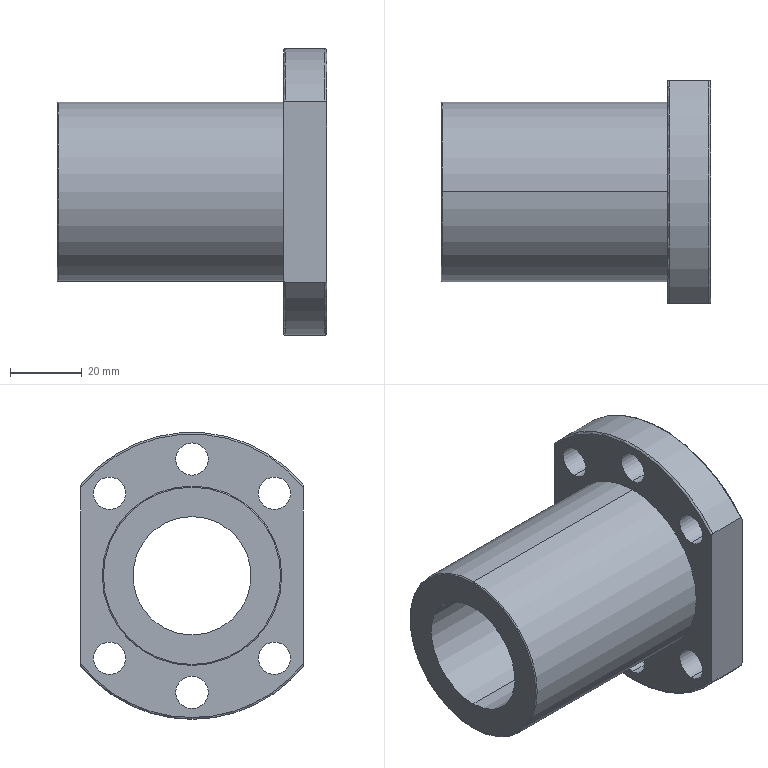Part | SolidWorks | features Fillet 2, HoleWzd 2, Extrusion 1, Revolution 1 | 1 solid | 35 faces | box 75 x 62 x 80 mm | volume 102466 mm3 | cylinder 21 | torus 8 | plane 6 | commonest cylinder face diameters 9 x12 80 x3 33 x2 49.5 x2 50 x2
STEP:
#1=CARTESIAN_POINT('',(-31.893,-0.000000261,-39.5));
#2=VERTEX_POINT('',#1);
#3=CARTESIAN_POINT('',(-31.893,-31.,-24.48));
#4=VERTEX_POINT('',#3);
#5=CARTESIAN_POINT('',(-31.893,-0.000000261,0.));
#6=DIRECTION('',(-1.,0.,0.));
#7=DIRECTION('',(0.,0.,-1.));
#8=AXIS2_PLACEMENT_3D('',#5,#6,#7);
#9=CIRCLE('',#8,39.5);
#10=EDGE_CURVE('',#2,#4,#9,.T.);
#11=ORIENTED_EDGE('',*,*,#10,.F.);
#12=CARTESIAN_POINT('',(-31.393,-0.000000261,-40.));
#13=VERTEX_POINT('',#12);
#14=CARTESIAN_POINT('',(-31.393,-0.000000261,-39.5));
#15=DIRECTION('',(0.,-1.,0.));
#16=DIRECTION('',(0.,0.,-1.));
#17=AXIS2_PLACEMENT_3D('',#14,#15,#16);
#18=CIRCLE('',#17,0.5);
#19=EDGE_CURVE('',#2,#13,#18,.T.);
#20=ORIENTED_EDGE('',*,*,#19,.T.);
#21=CARTESIAN_POINT('',(-31.393,-31.,-25.278));
#22=VERTEX_POINT('',#21);
#23=CARTESIAN_POINT('',(-31.393,-0.000000261,0.));
#24=DIRECTION('',(1.,0.,0.));
#25=DIRECTION('',(0.,0.,-1.));
#26=AXIS2_PLACEMENT_3D('',#23,#24,#25);
#27=CIRCLE('',#26,40.);
#28=EDGE_CURVE('',#22,#13,#27,.T.);
#29=ORIENTED_EDGE('',*,*,#28,.F.);
#30=CARTESIAN_POINT('',(-31.893,-31.,-24.48));
#31=CARTESIAN_POINT('',(-31.893,-31.,-24.566));
#32=CARTESIAN_POINT('',(-31.885,-31.,-24.651));
#33=CARTESIAN_POINT('',(-31.85,-31.,-24.818));
#34=CARTESIAN_POINT('',(-31.823,-31.,-24.901));
#35=CARTESIAN_POINT('',(-31.746,-31.,-25.056));
#36=CARTESIAN_POINT('',(-31.695,-31.,-25.128));
#37=CARTESIAN_POINT('',(-31.564,-31.,-25.24));
#38=CARTESIAN_POINT('',(-31.481,-31.,-25.278));
#39=CARTESIAN_POINT('',(-31.393,-31.,-25.278));
#40=B_SPLINE_CURVE_WITH_KNOTS('',3,(#30,#31,#32,#33,#34,#35,#36,#37,#38,#39),.UNSPECIFIED.,.F.,.F.,(4,2,2,2,4),(0.,0.0002558,0.0005116,0.0007674,0.001023),.UNSPECIFIED.);
#41=EDGE_CURVE('',#4,#22,#40,.T.);
#42=ORIENTED_EDGE('',*,*,#41,.F.);
#43=EDGE_LOOP('',(#11,#20,#29,#42));
#44=FACE_OUTER_BOUND('',#43,.T.);
#45=CARTESIAN_POINT('',(-31.393,-0.000000261,0.));
#46=DIRECTION('',(1.,0.,0.));
#47=DIRECTION('',(0.,0.,-1.));
#48=AXIS2_PLACEMENT_3D('',#45,#46,#47);
#49=TOROIDAL_SURFACE('',#48,39.5,0.5);
#50=ADVANCED_FACE('',(#44),#49,.T.);
#51=CARTESIAN_POINT('',(-20.393,-0.000000261,-40.));
#52=VERTEX_POINT('',#51);
#53=CARTESIAN_POINT('',(-20.393,-31.,-25.278));
#54=VERTEX_POINT('',#53);
#55=CARTESIAN_POINT('',(-20.393,-0.000000261,0.));
#56=DIRECTION('',(-1.,0.,0.));
#57=DIRECTION('',(0.,0.,-1.));
#58=AXIS2_PLACEMENT_3D('',#55,#56,#57);
#59=CIRCLE('',#58,40.);
#60=EDGE_CURVE('',#52,#54,#59,.T.);
#61=ORIENTED_EDGE('',*,*,#60,.F.);
#62=CARTESIAN_POINT('',(-19.893,-0.000000261,-39.5));
#63=VERTEX_POINT('',#62);
#64=CARTESIAN_POINT('',(-20.393,-0.000000261,-39.5));
#65=DIRECTION('',(0.,-1.,0.));
#66=DIRECTION('',(0.,0.,-1.));
#67=AXIS2_PLACEMENT_3D('',#64,#65,#66);
#68=CIRCLE('',#67,0.5);
#69=EDGE_CURVE('',#52,#63,#68,.T.);
#70=ORIENTED_EDGE('',*,*,#69,.T.);
#71=CARTESIAN_POINT('',(-19.893,-31.,-24.48));
#72=VERTEX_POINT('',#71);
#73=CARTESIAN_POINT('',(-19.893,-0.000000261,0.));
#74=DIRECTION('',(1.,0.,0.));
#75=DIRECTION('',(0.,0.,-1.));
#76=AXIS2_PLACEMENT_3D('',#73,#74,#75);
#77=CIRCLE('',#76,39.5);
#78=EDGE_CURVE('',#72,#63,#77,.T.);
#79=ORIENTED_EDGE('',*,*,#78,.F.);
#80=CARTESIAN_POINT('',(-20.393,-31.,-25.278));
#81=CARTESIAN_POINT('',(-20.306,-31.,-25.278));
#82=CARTESIAN_POINT('',(-20.223,-31.,-25.241));
#83=CARTESIAN_POINT('',(-20.091,-31.,-25.128));
#84=CARTESIAN_POINT('',(-20.04,-31.,-25.056));
#85=CARTESIAN_POINT('',(-19.925,-31.,-24.826));
#86=CARTESIAN_POINT('',(-19.893,-31.,-24.653));
#87=CARTESIAN_POINT('',(-19.893,-31.,-24.48));
#88=B_SPLINE_CURVE_WITH_KNOTS('',3,(#80,#81,#82,#83,#84,#85,#86,#87),.UNSPECIFIED.,.F.,.F.,(4,2,2,4),(0.,0.0002576,0.0005153,0.001031),.UNSPECIFIED.);
#89=EDGE_CURVE('',#54,#72,#88,.T.);
#90=ORIENTED_EDGE('',*,*,#89,.F.);
#91=EDGE_LOOP('',(#61,#70,#79,#90));
#92=FACE_OUTER_BOUND('',#91,.T.);
#93=CARTESIAN_POINT('',(-20.393,-0.000000261,0.));
#94=DIRECTION('',(1.,0.,0.));
#95=DIRECTION('',(0.,0.,-1.));
#96=AXIS2_PLACEMENT_3D('',#93,#94,#95);
#97=TOROIDAL_SURFACE('',#96,39.5,0.5);
#98=ADVANCED_FACE('',(#92),#97,.T.);
#99=CARTESIAN_POINT('',(-94.593,-0.000001246,-25.));
#100=VERTEX_POINT('',#99);
#101=CARTESIAN_POINT('',(-94.593,-0.000001246,25.));
#102=VERTEX_POINT('',#101);
#103=CARTESIAN_POINT('',(-94.593,-0.000001246,0.));
#104=DIRECTION('',(1.,0.,0.));
#105=DIRECTION('',(0.,0.,1.));
#106=AXIS2_PLACEMENT_3D('',#103,#104,#105);
#107=CIRCLE('',#106,25.);
#108=EDGE_CURVE('',#100,#102,#107,.T.);
#109=ORIENTED_EDGE('',*,*,#108,.F.);
#110=CARTESIAN_POINT('',(-94.893,-0.000001246,-24.7));
#111=VERTEX_POINT('',#110);
#112=CARTESIAN_POINT('',(-94.593,-0.000001246,-24.7));
#113=DIRECTION('',(0.,1.,0.));
#114=DIRECTION('',(0.,0.,1.));
#115=AXIS2_PLACEMENT_3D('',#112,#113,#114);
#116=CIRCLE('',#115,0.3);
#117=EDGE_CURVE('',#100,#111,#116,.T.);
#118=ORIENTED_EDGE('',*,*,#117,.T.);
#119=CARTESIAN_POINT('',(-94.893,-0.000001246,24.7));
#120=VERTEX_POINT('',#119);
#121=CARTESIAN_POINT('',(-94.893,-0.000001246,0.));
#122=DIRECTION('',(-1.,0.,0.));
#123=DIRECTION('',(0.,0.,1.));
#124=AXIS2_PLACEMENT_3D('',#121,#122,#123);
#125=CIRCLE('',#124,24.7);
#126=EDGE_CURVE('',#120,#111,#125,.T.);
#127=ORIENTED_EDGE('',*,*,#126,.F.);
#128=CARTESIAN_POINT('',(-94.593,-0.000001246,24.7));
#129=DIRECTION('',(0.,-1.,0.));
#130=DIRECTION('',(0.,0.,-1.));
#131=AXIS2_PLACEMENT_3D('',#128,#129,#130);
#132=CIRCLE('',#131,0.3);
#133=EDGE_CURVE('',#102,#120,#132,.T.);
#134=ORIENTED_EDGE('',*,*,#133,.F.);
#135=EDGE_LOOP('',(#109,#118,#127,#134));
#136=FACE_OUTER_BOUND('',#135,.T.);
#137=CARTESIAN_POINT('',(-94.593,-0.000001246,0.));
#138=DIRECTION('',(-1.,0.,0.));
#139=DIRECTION('',(0.,0.,1.));
#140=AXIS2_PLACEMENT_3D('',#137,#138,#139);
#141=TOROIDAL_SURFACE('',#140,24.7,0.3);
#142=ADVANCED_FACE('',(#136),#141,.T.);
#143=CARTESIAN_POINT('',(-24.893,-0.000000261,24.75));
#144=VERTEX_POINT('',#143);
#145=CARTESIAN_POINT('',(-24.893,-0.000000261,-24.75));
#146=VERTEX_POINT('',#145);
#147=CARTESIAN_POINT('',(-24.893,-0.000000261,0.));
#148=DIRECTION('',(1.,0.,0.));
#149=DIRECTION('',(0.,0.,-1.));
#150=AXIS2_PLACEMENT_3D('',#147,#148,#149);
#151=CIRCLE('',#150,24.75);
#152=EDGE_CURVE('',#144,#146,#151,.T.);
#153=ORIENTED_EDGE('',*,*,#152,.F.);
#154=CARTESIAN_POINT('',(-19.893,-0.000000261,24.75));
#155=VERTEX_POINT('',#154);
#156=CARTESIAN_POINT('',(-19.893,-0.000000261,24.75));
#157=DIRECTION('',(1.,0.,0.));
#158=VECTOR('',#157,1000.);
#159=LINE('',#156,#158);
#160=EDGE_CURVE('',#144,#155,#159,.T.);
#161=ORIENTED_EDGE('',*,*,#160,.T.);
#162=CARTESIAN_POINT('',(-19.893,-0.000000261,-24.75));
#163=VERTEX_POINT('',#162);
#164=CARTESIAN_POINT('',(-19.893,-0.000000261,0.));
#165=DIRECTION('',(1.,0.,0.));
#166=DIRECTION('',(0.,0.,-1.));
#167=AXIS2_PLACEMENT_3D('',#164,#165,#166);
#168=CIRCLE('',#167,24.75);
#169=EDGE_CURVE('',#155,#163,#168,.T.);
#170=ORIENTED_EDGE('',*,*,#169,.T.);
#171=CARTESIAN_POINT('',(-19.893,-0.000000261,-24.75));
#172=DIRECTION('',(1.,0.,0.));
#173=VECTOR('',#172,1000.);
#174=LINE('',#171,#173);
#175=EDGE_CURVE('',#146,#163,#174,.T.);
#176=ORIENTED_EDGE('',*,*,#175,.F.);
#177=EDGE_LOOP('',(#153,#161,#170,#176));
#178=FACE_OUTER_BOUND('',#177,.T.);
#179=CARTESIAN_POINT('',(-19.893,-0.000000261,0.));
#180=DIRECTION('',(1.,0.,0.));
#181=DIRECTION('',(0.,0.,-1.));
#182=AXIS2_PLACEMENT_3D('',#179,#180,#181);
#183=CYLINDRICAL_SURFACE('',#182,24.75);
#184=ADVANCED_FACE('',(#178),#183,.F.);
#185=CARTESIAN_POINT('',(-94.893,-0.000000261,16.5));
#186=VERTEX_POINT('',#185);
#187=CARTESIAN_POINT('',(-94.893,-0.000000261,-16.5));
#188=VERTEX_POINT('',#187);
#189=CARTESIAN_POINT('',(-94.893,-0.000000261,0.));
#190=DIRECTION('',(1.,0.,0.));
#191=DIRECTION('',(0.,0.,-1.));
#192=AXIS2_PLACEMENT_3D('',#189,#190,#191);
#193=CIRCLE('',#192,16.5);
#194=EDGE_CURVE('',#186,#188,#193,.T.);
#195=ORIENTED_EDGE('',*,*,#194,.F.);
#196=CARTESIAN_POINT('',(-24.893,-0.000000261,16.5));
#197=VERTEX_POINT('',#196);
#198=CARTESIAN_POINT('',(-19.893,-0.000000261,16.5));
#199=DIRECTION('',(1.,0.,0.));
#200=VECTOR('',#199,1000.);
#201=LINE('',#198,#200);
#202=EDGE_CURVE('',#186,#197,#201,.T.);
#203=ORIENTED_EDGE('',*,*,#202,.T.);
#204=CARTESIAN_POINT('',(-24.893,-0.000000261,-16.5));
#205=VERTEX_POINT('',#204);
#206=CARTESIAN_POINT('',(-24.893,-0.000000261,0.));
#207=DIRECTION('',(1.,0.,0.));
#208=DIRECTION('',(0.,0.,-1.));
#209=AXIS2_PLACEMENT_3D('',#206,#207,#208);
#210=CIRCLE('',#209,16.5);
#211=EDGE_CURVE('',#197,#205,#210,.T.);
#212=ORIENTED_EDGE('',*,*,#211,.T.);
#213=CARTESIAN_POINT('',(-19.893,-0.000000261,-16.5));
#214=DIRECTION('',(1.,0.,0.));
#215=VECTOR('',#214,1000.);
#216=LINE('',#213,#215);
#217=EDGE_CURVE('',#188,#205,#216,.T.);
#218=ORIENTED_EDGE('',*,*,#217,.F.);
#219=EDGE_LOOP('',(#195,#203,#212,#218));
#220=FACE_OUTER_BOUND('',#219,.T.);
#221=CARTESIAN_POINT('',(-19.893,-0.000000261,0.));
#222=DIRECTION('',(1.,0.,0.));
#223=DIRECTION('',(0.,0.,-1.));
#224=AXIS2_PLACEMENT_3D('',#221,#222,#223);
#225=CYLINDRICAL_SURFACE('',#224,16.5);
#226=ADVANCED_FACE('',(#220),#225,.F.);
#227=CARTESIAN_POINT('',(-19.893,22.981,18.481));
#228=VERTEX_POINT('',#227);
#229=CARTESIAN_POINT('',(-19.893,22.981,27.481));
#230=VERTEX_POINT('',#229);
#231=CARTESIAN_POINT('',(-19.893,22.981,22.981));
#232=DIRECTION('',(-1.,0.,0.));
#233=DIRECTION('',(0.,0.,1.));
#234=AXIS2_PLACEMENT_3D('',#231,#232,#233);
#235=CIRCLE('',#234,4.5);
#236=EDGE_CURVE('',#228,#230,#235,.T.);
#237=ORIENTED_EDGE('',*,*,#236,.F.);
#238=CARTESIAN_POINT('',(-31.893,22.981,18.481));
#239=VERTEX_POINT('',#238);
#240=CARTESIAN_POINT('',(-31.893,22.981,18.481));
#241=DIRECTION('',(-1.,0.,0.));
#242=VECTOR('',#241,1000.);
#243=LINE('',#240,#242);
#244=EDGE_CURVE('',#228,#239,#243,.T.);
#245=ORIENTED_EDGE('',*,*,#244,.T.);
#246=CARTESIAN_POINT('',(-31.893,22.981,27.481));
#247=VERTEX_POINT('',#246);
#248=CARTESIAN_POINT('',(-31.893,22.981,22.981));
#249=DIRECTION('',(-1.,0.,0.));
#250=DIRECTION('',(0.,0.,1.));
#251=AXIS2_PLACEMENT_3D('',#248,#249,#250);
#252=CIRCLE('',#251,4.5);
#253=EDGE_CURVE('',#239,#247,#252,.T.);
#254=ORIENTED_EDGE('',*,*,#253,.T.);
#255=CARTESIAN_POINT('',(-31.893,22.981,27.481));
#256=DIRECTION('',(-1.,0.,0.));
#257=VECTOR('',#256,1000.);
#258=LINE('',#255,#257);
#259=EDGE_CURVE('',#230,#247,#258,.T.);
#260=ORIENTED_EDGE('',*,*,#259,.F.);
#261=EDGE_LOOP('',(#237,#245,#254,#260));
#262=FACE_OUTER_BOUND('',#261,.T.);
#263=CARTESIAN_POINT('',(-31.893,22.981,22.981));
#264=DIRECTION('',(-1.,0.,0.));
#265=DIRECTION('',(0.,0.,1.));
#266=AXIS2_PLACEMENT_3D('',#263,#264,#265);
#267=CYLINDRICAL_SURFACE('',#266,4.5);
#268=ADVANCED_FACE('',(#262),#267,.F.);
#269=CARTESIAN_POINT('',(-19.893,-22.981,18.481));
#270=VERTEX_POINT('',#269);
#271=CARTESIAN_POINT('',(-19.893,-22.981,27.481));
#272=VERTEX_POINT('',#271);
#273=CARTESIAN_POINT('',(-19.893,-22.981,22.981));
#274=DIRECTION('',(-1.,0.,0.));
#275=DIRECTION('',(0.,0.,1.));
#276=AXIS2_PLACEMENT_3D('',#273,#274,#275);
#277=CIRCLE('',#276,4.5);
#278=EDGE_CURVE('',#270,#272,#277,.T.);
#279=ORIENTED_EDGE('',*,*,#278,.F.);
#280=CARTESIAN_POINT('',(-31.893,-22.981,18.481));
#281=VERTEX_POINT('',#280);
#282=CARTESIAN_POINT('',(-31.893,-22.981,18.481));
#283=DIRECTION('',(-1.,0.,0.));
#284=VECTOR('',#283,1000.);
#285=LINE('',#282,#284);
#286=EDGE_CURVE('',#270,#281,#285,.T.);
#287=ORIENTED_EDGE('',*,*,#286,.T.);
#288=CARTESIAN_POINT('',(-31.893,-22.981,27.481));
#289=VERTEX_POINT('',#288);
#290=CARTESIAN_POINT('',(-31.893,-22.981,22.981));
#291=DIRECTION('',(-1.,0.,0.));
#292=DIRECTION('',(0.,0.,1.));
#293=AXIS2_PLACEMENT_3D('',#290,#291,#292);
#294=CIRCLE('',#293,4.5);
#295=EDGE_CURVE('',#281,#289,#294,.T.);
#296=ORIENTED_EDGE('',*,*,#295,.T.);
#297=CARTESIAN_POINT('',(-31.893,-22.981,27.481));
#298=DIRECTION('',(-1.,0.,0.));
#299=VECTOR('',#298,1000.);
#300=LINE('',#297,#299);
#301=EDGE_CURVE('',#272,#289,#300,.T.);
#302=ORIENTED_EDGE('',*,*,#301,.F.);
#303=EDGE_LOOP('',(#279,#287,#296,#302));
#304=FACE_OUTER_BOUND('',#303,.T.);
#305=CARTESIAN_POINT('',(-31.893,-22.981,22.981));
#306=DIRECTION('',(-1.,0.,0.));
#307=DIRECTION('',(0.,0.,1.));
#308=AXIS2_PLACEMENT_3D('',#305,#306,#307);
#309=CYLINDRICAL_SURFACE('',#308,4.5);
#310=ADVANCED_FACE('',(#304),#309,.F.);
#311=CARTESIAN_POINT('',(-19.893,-22.981,-27.481));
#312=VERTEX_POINT('',#311);
#313=CARTESIAN_POINT('',(-19.893,-22.981,-18.481));
#314=VERTEX_POINT('',#313);
#315=CARTESIAN_POINT('',(-19.893,-22.981,-22.981));
#316=DIRECTION('',(-1.,0.,0.));
#317=DIRECTION('',(0.,0.,1.));
#318=AXIS2_PLACEMENT_3D('',#315,#316,#317);
#319=CIRCLE('',#318,4.5);
#320=EDGE_CURVE('',#312,#314,#319,.T.);
#321=ORIENTED_EDGE('',*,*,#320,.F.);
#322=CARTESIAN_POINT('',(-31.893,-22.981,-27.481));
#323=VERTEX_POINT('',#322);
#324=CARTESIAN_POINT('',(-31.893,-22.981,-27.481));
#325=DIRECTION('',(-1.,0.,0.));
#326=VECTOR('',#325,1000.);
#327=LINE('',#324,#326);
#328=EDGE_CURVE('',#312,#323,#327,.T.);
#329=ORIENTED_EDGE('',*,*,#328,.T.);
#330=CARTESIAN_POINT('',(-31.893,-22.981,-18.481));
#331=VERTEX_POINT('',#330);
#332=CARTESIAN_POINT('',(-31.893,-22.981,-22.981));
#333=DIRECTION('',(-1.,0.,0.));
#334=DIRECTION('',(0.,0.,1.));
#335=AXIS2_PLACEMENT_3D('',#332,#333,#334);
#336=CIRCLE('',#335,4.5);
#337=EDGE_CURVE('',#323,#331,#336,.T.);
#338=ORIENTED_EDGE('',*,*,#337,.T.);
#339=CARTESIAN_POINT('',(-31.893,-22.981,-18.481));
#340=DIRECTION('',(-1.,0.,0.));
#341=VECTOR('',#340,1000.);
#342=LINE('',#339,#341);
#343=EDGE_CURVE('',#314,#331,#342,.T.);
#344=ORIENTED_EDGE('',*,*,#343,.F.);
#345=EDGE_LOOP('',(#321,#329,#338,#344));
#346=FACE_OUTER_BOUND('',#345,.T.);
#347=CARTESIAN_POINT('',(-31.893,-22.981,-22.981));
#348=DIRECTION('',(-1.,0.,0.));
#349=DIRECTION('',(0.,0.,1.));
#350=AXIS2_PLACEMENT_3D('',#347,#348,#349);
#351=CYLINDRICAL_SURFACE('',#350,4.5);
#352=ADVANCED_FACE('',(#346),#351,.F.);
#353=CARTESIAN_POINT('',(-19.893,22.981,-27.481));
#354=VERTEX_POINT('',#353);
#355=CARTESIAN_POINT('',(-19.893,22.981,-18.481));
#356=VERTEX_POINT('',#355);
#357=CARTESIAN_POINT('',(-19.893,22.981,-22.981));
#358=DIRECTION('',(-1.,0.,0.));
#359=DIRECTION('',(0.,0.,1.));
#360=AXIS2_PLACEMENT_3D('',#357,#358,#359);
#361=CIRCLE('',#360,4.5);
#362=EDGE_CURVE('',#354,#356,#361,.T.);
#363=ORIENTED_EDGE('',*,*,#362,.F.);
#364=CARTESIAN_POINT('',(-31.893,22.981,-27.481));
#365=VERTEX_POINT('',#364);
#366=CARTESIAN_POINT('',(-31.893,22.981,-27.481));
#367=DIRECTION('',(-1.,0.,0.));
#368=VECTOR('',#367,1000.);
#369=LINE('',#366,#368);
#370=EDGE_CURVE('',#354,#365,#369,.T.);
#371=ORIENTED_EDGE('',*,*,#370,.T.);
#372=CARTESIAN_POINT('',(-31.893,22.981,-18.481));
#373=VERTEX_POINT('',#372);
#374=CARTESIAN_POINT('',(-31.893,22.981,-22.981));
#375=DIRECTION('',(-1.,0.,0.));
#376=DIRECTION('',(0.,0.,1.));
#377=AXIS2_PLACEMENT_3D('',#374,#375,#376);
#378=CIRCLE('',#377,4.5);
#379=EDGE_CURVE('',#365,#373,#378,.T.);
#380=ORIENTED_EDGE('',*,*,#379,.T.);
#381=CARTESIAN_POINT('',(-31.893,22.981,-18.481));
#382=DIRECTION('',(-1.,0.,0.));
#383=VECTOR('',#382,1000.);
#384=LINE('',#381,#383);
#385=EDGE_CURVE('',#356,#373,#384,.T.);
#386=ORIENTED_EDGE('',*,*,#385,.F.);
#387=EDGE_LOOP('',(#363,#371,#380,#386));
#388=FACE_OUTER_BOUND('',#387,.T.);
#389=CARTESIAN_POINT('',(-31.893,22.981,-22.981));
#390=DIRECTION('',(-1.,0.,0.));
#391=DIRECTION('',(0.,0.,1.));
#392=AXIS2_PLACEMENT_3D('',#389,#390,#391);
#393=CYLINDRICAL_SURFACE('',#392,4.5);
#394=ADVANCED_FACE('',(#388),#393,.F.);
#395=CARTESIAN_POINT('',(-19.893,-0.000000419,28.));
#396=VERTEX_POINT('',#395);
#397=CARTESIAN_POINT('',(-19.893,-0.000000419,37.));
#398=VERTEX_POINT('',#397);
#399=CARTESIAN_POINT('',(-19.893,-0.000000419,32.5));
#400=DIRECTION('',(-1.,0.,0.));
#401=DIRECTION('',(0.,0.,1.));
#402=AXIS2_PLACEMENT_3D('',#399,#400,#401);
#403=CIRCLE('',#402,4.5);
#404=EDGE_CURVE('',#396,#398,#403,.T.);
#405=ORIENTED_EDGE('',*,*,#404,.F.);
#406=CARTESIAN_POINT('',(-31.893,-0.000000419,28.));
#407=VERTEX_POINT('',#406);
#408=CARTESIAN_POINT('',(-31.893,-0.000000419,28.));
#409=DIRECTION('',(-1.,0.,0.));
#410=VECTOR('',#409,1000.);
#411=LINE('',#408,#410);
#412=EDGE_CURVE('',#396,#407,#411,.T.);
#413=ORIENTED_EDGE('',*,*,#412,.T.);
#414=CARTESIAN_POINT('',(-31.893,-0.000000419,37.));
#415=VERTEX_POINT('',#414);
#416=CARTESIAN_POINT('',(-31.893,-0.000000419,32.5));
#417=DIRECTION('',(-1.,0.,0.));
#418=DIRECTION('',(0.,0.,1.));
#419=AXIS2_PLACEMENT_3D('',#416,#417,#418);
#420=CIRCLE('',#419,4.5);
#421=EDGE_CURVE('',#407,#415,#420,.T.);
#422=ORIENTED_EDGE('',*,*,#421,.T.);
#423=CARTESIAN_POINT('',(-31.893,-0.000000419,37.));
#424=DIRECTION('',(-1.,0.,0.));
#425=VECTOR('',#424,1000.);
#426=LINE('',#423,#425);
#427=EDGE_CURVE('',#398,#415,#426,.T.);
#428=ORIENTED_EDGE('',*,*,#427,.F.);
#429=EDGE_LOOP('',(#405,#413,#422,#428));
#430=FACE_OUTER_BOUND('',#429,.T.);
#431=CARTESIAN_POINT('',(-31.893,-0.000000419,32.5));
#432=DIRECTION('',(-1.,0.,0.));
#433=DIRECTION('',(0.,0.,1.));
#434=AXIS2_PLACEMENT_3D('',#431,#432,#433);
#435=CYLINDRICAL_SURFACE('',#434,4.5);
#436=ADVANCED_FACE('',(#430),#435,.F.);
#437=CARTESIAN_POINT('',(-19.893,-0.000000419,-37.));
#438=VERTEX_POINT('',#437);
#439=CARTESIAN_POINT('',(-19.893,-0.000000419,-28.));
#440=VERTEX_POINT('',#439);
#441=CARTESIAN_POINT('',(-19.893,-0.000000419,-32.5));
#442=DIRECTION('',(-1.,0.,0.));
#443=DIRECTION('',(0.,0.,1.));
#444=AXIS2_PLACEMENT_3D('',#441,#442,#443);
#445=CIRCLE('',#444,4.5);
#446=EDGE_CURVE('',#438,#440,#445,.T.);
#447=ORIENTED_EDGE('',*,*,#446,.F.);
#448=CARTESIAN_POINT('',(-31.893,-0.000000419,-37.));
#449=VERTEX_POINT('',#448);
#450=CARTESIAN_POINT('',(-31.893,-0.000000419,-37.));
#451=DIRECTION('',(-1.,0.,0.));
#452=VECTOR('',#451,1000.);
#453=LINE('',#450,#452);
#454=EDGE_CURVE('',#438,#449,#453,.T.);
#455=ORIENTED_EDGE('',*,*,#454,.T.);
#456=CARTESIAN_POINT('',(-31.893,-0.000000419,-28.));
#457=VERTEX_POINT('',#456);
#458=CARTESIAN_POINT('',(-31.893,-0.000000419,-32.5));
#459=DIRECTION('',(-1.,0.,0.));
#460=DIRECTION('',(0.,0.,1.));
#461=AXIS2_PLACEMENT_3D('',#458,#459,#460);
#462=CIRCLE('',#461,4.5);
#463=EDGE_CURVE('',#449,#457,#462,.T.);
#464=ORIENTED_EDGE('',*,*,#463,.T.);
#465=CARTESIAN_POINT('',(-31.893,-0.000000419,-28.));
#466=DIRECTION('',(-1.,0.,0.));
#467=VECTOR('',#466,1000.);
#468=LINE('',#465,#467);
#469=EDGE_CURVE('',#440,#457,#468,.T.);
#470=ORIENTED_EDGE('',*,*,#469,.F.);
#471=EDGE_LOOP('',(#447,#455,#464,#470));
#472=FACE_OUTER_BOUND('',#471,.T.);
#473=CARTESIAN_POINT('',(-31.893,-0.000000419,-32.5));
#474=DIRECTION('',(-1.,0.,0.));
#475=DIRECTION('',(0.,0.,1.));
#476=AXIS2_PLACEMENT_3D('',#473,#474,#475);
#477=CYLINDRICAL_SURFACE('',#476,4.5);
#478=ADVANCED_FACE('',(#472),#477,.F.);
#479=ORIENTED_EDGE('',*,*,#108,.T.);
#480=CARTESIAN_POINT('',(-31.893,-0.000001246,25.));
#481=VERTEX_POINT('',#480);
#482=CARTESIAN_POINT('',(-94.893,-0.000001246,25.));
#483=DIRECTION('',(1.,0.,0.));
#484=VECTOR('',#483,1000.);
#485=LINE('',#482,#484);
#486=EDGE_CURVE('',#102,#481,#485,.T.);
#487=ORIENTED_EDGE('',*,*,#486,.T.);
#488=CARTESIAN_POINT('',(-31.893,-0.000001246,-25.));
#489=VERTEX_POINT('',#488);
#490=CARTESIAN_POINT('',(-31.893,-0.000001246,0.));
#491=DIRECTION('',(1.,0.,0.));
#492=DIRECTION('',(0.,0.,-1.));
#493=AXIS2_PLACEMENT_3D('',#490,#491,#492);
#494=CIRCLE('',#493,25.);
#495=EDGE_CURVE('',#489,#481,#494,.T.);
#496=ORIENTED_EDGE('',*,*,#495,.F.);
#497=CARTESIAN_POINT('',(-94.893,-0.000001246,-25.));
#498=DIRECTION('',(1.,0.,0.));
#499=VECTOR('',#498,1000.);
#500=LINE('',#497,#499);
#501=EDGE_CURVE('',#100,#489,#500,.T.);
#502=ORIENTED_EDGE('',*,*,#501,.F.);
#503=EDGE_LOOP('',(#479,#487,#496,#502));
#504=FACE_OUTER_BOUND('',#503,.T.);
#505=CARTESIAN_POINT('',(-94.893,-0.000001246,0.));
#506=DIRECTION('',(1.,0.,0.));
#507=DIRECTION('',(0.,0.,-1.));
#508=AXIS2_PLACEMENT_3D('',#505,#506,#507);
#509=CYLINDRICAL_SURFACE('',#508,25.);
#510=ADVANCED_FACE('',(#504),#509,.T.);
#511=ORIENTED_EDGE('',*,*,#28,.T.);
#512=CARTESIAN_POINT('',(-31.893,-0.000000261,-40.));
#513=DIRECTION('',(1.,0.,0.));
#514=VECTOR('',#513,1000.);
#515=LINE('',#512,#514);
#516=EDGE_CURVE('',#13,#52,#515,.T.);
#517=ORIENTED_EDGE('',*,*,#516,.T.);
#518=ORIENTED_EDGE('',*,*,#60,.T.);
#519=CARTESIAN_POINT('',(-31.893,-31.,-25.278));
#520=DIRECTION('',(1.,0.,0.));
#521=VECTOR('',#520,1000.);
#522=LINE('',#519,#521);
#523=EDGE_CURVE('',#22,#54,#522,.T.);
#524=ORIENTED_EDGE('',*,*,#523,.F.);
#525=EDGE_LOOP('',(#511,#517,#518,#524));
#526=FACE_OUTER_BOUND('',#525,.T.);
#527=CARTESIAN_POINT('',(-31.893,-0.000000261,0.));
#528=DIRECTION('',(1.,0.,0.));
#529=DIRECTION('',(0.,0.,-1.));
#530=AXIS2_PLACEMENT_3D('',#527,#528,#529);
#531=CYLINDRICAL_SURFACE('',#530,40.);
#532=ADVANCED_FACE('',(#526),#531,.T.);
#533=ORIENTED_EDGE('',*,*,#516,.F.);
#534=CARTESIAN_POINT('',(-31.393,31.,-25.278));
#535=VERTEX_POINT('',#534);
#536=CARTESIAN_POINT('',(-31.393,-0.000000261,0.));
#537=DIRECTION('',(1.,0.,0.));
#538=DIRECTION('',(0.,0.,-1.));
#539=AXIS2_PLACEMENT_3D('',#536,#537,#538);
#540=CIRCLE('',#539,40.);
#541=EDGE_CURVE('',#13,#535,#540,.T.);
#542=ORIENTED_EDGE('',*,*,#541,.T.);
#543=CARTESIAN_POINT('',(-20.393,31.,-25.278));
#544=VERTEX_POINT('',#543);
#545=CARTESIAN_POINT('',(-31.893,31.,-25.278));
#546=DIRECTION('',(1.,0.,0.));
#547=VECTOR('',#546,1000.);
#548=LINE('',#545,#547);
#549=EDGE_CURVE('',#535,#544,#548,.T.);
#550=ORIENTED_EDGE('',*,*,#549,.T.);
#551=CARTESIAN_POINT('',(-20.393,-0.000000261,0.));
#552=DIRECTION('',(-1.,0.,0.));
#553=DIRECTION('',(0.,0.,-1.));
#554=AXIS2_PLACEMENT_3D('',#551,#552,#553);
#555=CIRCLE('',#554,40.);
#556=EDGE_CURVE('',#544,#52,#555,.T.);
#557=ORIENTED_EDGE('',*,*,#556,.T.);
#558=EDGE_LOOP('',(#533,#542,#550,#557));
#559=FACE_OUTER_BOUND('',#558,.T.);
#560=CARTESIAN_POINT('',(-31.893,-0.000000261,0.));
#561=DIRECTION('',(1.,0.,0.));
#562=DIRECTION('',(0.,0.,-1.));
#563=AXIS2_PLACEMENT_3D('',#560,#561,#562);
#564=CYLINDRICAL_SURFACE('',#563,40.);
#565=ADVANCED_FACE('',(#559),#564,.T.);
#566=CARTESIAN_POINT('',(-31.393,-31.,25.278));
#567=VERTEX_POINT('',#566);
#568=CARTESIAN_POINT('',(-20.393,-31.,25.278));
#569=VERTEX_POINT('',#568);
#570=CARTESIAN_POINT('',(-31.893,-31.,25.278));
#571=DIRECTION('',(1.,0.,0.));
#572=VECTOR('',#571,1000.);
#573=LINE('',#570,#572);
#574=EDGE_CURVE('',#567,#569,#573,.T.);
#575=ORIENTED_EDGE('',*,*,#574,.F.);
#576=CARTESIAN_POINT('',(-31.893,-31.,24.48));
#577=VERTEX_POINT('',#576);
#578=CARTESIAN_POINT('',(-31.393,-31.,25.278));
#579=CARTESIAN_POINT('',(-31.481,-31.,25.278));
#580=CARTESIAN_POINT('',(-31.563,-31.,25.241));
#581=CARTESIAN_POINT('',(-31.695,-31.,25.128));
#582=CARTESIAN_POINT('',(-31.746,-31.,25.056));
#583=CARTESIAN_POINT('',(-31.861,-31.,24.826));
#584=CARTESIAN_POINT('',(-31.893,-31.,24.653));
#585=CARTESIAN_POINT('',(-31.893,-31.,24.48));
#586=B_SPLINE_CURVE_WITH_KNOTS('',3,(#578,#579,#580,#581,#582,#583,#584,#585),.UNSPECIFIED.,.F.,.F.,(4,2,2,4),(0.,0.0002576,0.0005153,0.001031),.UNSPECIFIED.);
#587=EDGE_CURVE('',#567,#577,#586,.T.);
#588=ORIENTED_EDGE('',*,*,#587,.T.);
#589=CARTESIAN_POINT('',(-31.893,-31.,25.278));
#590=DIRECTION('',(0.,0.,-1.));
#591=VECTOR('',#590,1000.);
#592=LINE('',#589,#591);
#593=EDGE_CURVE('',#577,#4,#592,.T.);
#594=ORIENTED_EDGE('',*,*,#593,.T.);
#595=ORIENTED_EDGE('',*,*,#41,.T.);
#596=ORIENTED_EDGE('',*,*,#523,.T.);
#597=ORIENTED_EDGE('',*,*,#89,.T.);
#598=CARTESIAN_POINT('',(-19.893,-31.,24.48));
#599=VERTEX_POINT('',#598);
#600=CARTESIAN_POINT('',(-19.893,-31.,25.278));
#601=DIRECTION('',(0.,0.,-1.));
#602=VECTOR('',#601,1000.);
#603=LINE('',#600,#602);
#604=EDGE_CURVE('',#599,#72,#603,.T.);
#605=ORIENTED_EDGE('',*,*,#604,.F.);
#606=CARTESIAN_POINT('',(-19.893,-31.,24.48));
#607=CARTESIAN_POINT('',(-19.893,-31.,24.566));
#608=CARTESIAN_POINT('',(-19.901,-31.,24.651));
#609=CARTESIAN_POINT('',(-19.936,-31.,24.818));
#610=CARTESIAN_POINT('',(-19.963,-31.,24.901));
#611=CARTESIAN_POINT('',(-20.04,-31.,25.056));
#612=CARTESIAN_POINT('',(-20.091,-31.,25.128));
#613=CARTESIAN_POINT('',(-20.222,-31.,25.24));
#614=CARTESIAN_POINT('',(-20.305,-31.,25.278));
#615=CARTESIAN_POINT('',(-20.393,-31.,25.278));
#616=B_SPLINE_CURVE_WITH_KNOTS('',3,(#606,#607,#608,#609,#610,#611,#612,#613,#614,#615),.UNSPECIFIED.,.F.,.F.,(4,2,2,2,4),(0.,0.0002558,0.0005116,0.0007674,0.001023),.UNSPECIFIED.);
#617=EDGE_CURVE('',#599,#569,#616,.T.);
#618=ORIENTED_EDGE('',*,*,#617,.T.);
#619=EDGE_LOOP('',(#575,#588,#594,#595,#596,#597,#605,#618));
#620=FACE_OUTER_BOUND('',#619,.T.);
#621=CARTESIAN_POINT('',(-31.893,-31.,25.278));
#622=DIRECTION('',(0.,-1.,0.));
#623=DIRECTION('',(0.,0.,-1.));
#624=AXIS2_PLACEMENT_3D('',#621,#622,#623);
#625=PLANE('',#624);
#626=ADVANCED_FACE('',(#620),#625,.T.);
#627=CARTESIAN_POINT('',(-31.393,31.,25.278));
#628=VERTEX_POINT('',#627);
#629=CARTESIAN_POINT('',(-20.393,31.,25.278));
#630=VERTEX_POINT('',#629);
#631=CARTESIAN_POINT('',(-31.893,31.,25.278));
#632=DIRECTION('',(1.,0.,0.));
#633=VECTOR('',#632,1000.);
#634=LINE('',#631,#633);
#635=EDGE_CURVE('',#628,#630,#634,.T.);
#636=ORIENTED_EDGE('',*,*,#635,.F.);
#637=CARTESIAN_POINT('',(-31.393,-0.000000261,0.));
#638=DIRECTION('',(1.,0.,0.));
#639=DIRECTION('',(0.,0.,-1.));
#640=AXIS2_PLACEMENT_3D('',#637,#638,#639);
#641=CIRCLE('',#640,40.);
#642=EDGE_CURVE('',#628,#567,#641,.T.);
#643=ORIENTED_EDGE('',*,*,#642,.T.);
#644=ORIENTED_EDGE('',*,*,#574,.T.);
#645=CARTESIAN_POINT('',(-20.393,-0.000000261,0.));
#646=DIRECTION('',(-1.,0.,0.));
#647=DIRECTION('',(0.,0.,-1.));
#648=AXIS2_PLACEMENT_3D('',#645,#646,#647);
#649=CIRCLE('',#648,40.);
#650=EDGE_CURVE('',#569,#630,#649,.T.);
#651=ORIENTED_EDGE('',*,*,#650,.T.);
#652=EDGE_LOOP('',(#636,#643,#644,#651));
#653=FACE_OUTER_BOUND('',#652,.T.);
#654=CARTESIAN_POINT('',(-31.893,-0.000000261,0.));
#655=DIRECTION('',(1.,0.,0.));
#656=DIRECTION('',(0.,0.,-1.));
#657=AXIS2_PLACEMENT_3D('',#654,#655,#656);
#658=CYLINDRICAL_SURFACE('',#657,40.);
#659=ADVANCED_FACE('',(#653),#658,.T.);
#660=CARTESIAN_POINT('',(-31.893,31.,-24.48));
#661=VERTEX_POINT('',#660);
#662=CARTESIAN_POINT('',(-31.893,31.,24.48));
#663=VERTEX_POINT('',#662);
#664=CARTESIAN_POINT('',(-31.893,31.,-25.278));
#665=DIRECTION('',(0.,0.,1.));
#666=VECTOR('',#665,1000.);
#667=LINE('',#664,#666);
#668=EDGE_CURVE('',#661,#663,#667,.T.);
#669=ORIENTED_EDGE('',*,*,#668,.T.);
#670=CARTESIAN_POINT('',(-31.893,31.,24.48));
#671=CARTESIAN_POINT('',(-31.893,31.,24.566));
#672=CARTESIAN_POINT('',(-31.885,31.,24.651));
#673=CARTESIAN_POINT('',(-31.85,31.,24.818));
#674=CARTESIAN_POINT('',(-31.823,31.,24.901));
#675=CARTESIAN_POINT('',(-31.746,31.,25.056));
#676=CARTESIAN_POINT('',(-31.695,31.,25.128));
#677=CARTESIAN_POINT('',(-31.564,31.,25.24));
#678=CARTESIAN_POINT('',(-31.481,31.,25.278));
#679=CARTESIAN_POINT('',(-31.393,31.,25.278));
#680=B_SPLINE_CURVE_WITH_KNOTS('',3,(#670,#671,#672,#673,#674,#675,#676,#677,#678,#679),.UNSPECIFIED.,.F.,.F.,(4,2,2,2,4),(0.,0.0002558,0.0005116,0.0007674,0.001023),.UNSPECIFIED.);
#681=EDGE_CURVE('',#663,#628,#680,.T.);
#682=ORIENTED_EDGE('',*,*,#681,.T.);
#683=ORIENTED_EDGE('',*,*,#635,.T.);
#684=CARTESIAN_POINT('',(-19.893,31.,24.48));
#685=VERTEX_POINT('',#684);
#686=CARTESIAN_POINT('',(-20.393,31.,25.278));
#687=CARTESIAN_POINT('',(-20.306,31.,25.278));
#688=CARTESIAN_POINT('',(-20.223,31.,25.241));
#689=CARTESIAN_POINT('',(-20.091,31.,25.128));
#690=CARTESIAN_POINT('',(-20.04,31.,25.056));
#691=CARTESIAN_POINT('',(-19.925,31.,24.826));
#692=CARTESIAN_POINT('',(-19.893,31.,24.653));
#693=CARTESIAN_POINT('',(-19.893,31.,24.48));
#694=B_SPLINE_CURVE_WITH_KNOTS('',3,(#686,#687,#688,#689,#690,#691,#692,#693),.UNSPECIFIED.,.F.,.F.,(4,2,2,4),(0.,0.0002576,0.0005153,0.001031),.UNSPECIFIED.);
#695=EDGE_CURVE('',#630,#685,#694,.T.);
#696=ORIENTED_EDGE('',*,*,#695,.T.);
#697=CARTESIAN_POINT('',(-19.893,31.,-24.48));
#698=VERTEX_POINT('',#697);
#699=CARTESIAN_POINT('',(-19.893,31.,-25.278));
#700=DIRECTION('',(0.,0.,1.));
#701=VECTOR('',#700,1000.);
#702=LINE('',#699,#701);
#703=EDGE_CURVE('',#698,#685,#702,.T.);
#704=ORIENTED_EDGE('',*,*,#703,.F.);
#705=CARTESIAN_POINT('',(-19.893,31.,-24.48));
#706=CARTESIAN_POINT('',(-19.893,31.,-24.566));
#707=CARTESIAN_POINT('',(-19.901,31.,-24.651));
#708=CARTESIAN_POINT('',(-19.936,31.,-24.818));
#709=CARTESIAN_POINT('',(-19.963,31.,-24.901));
#710=CARTESIAN_POINT('',(-20.04,31.,-25.056));
#711=CARTESIAN_POINT('',(-20.091,31.,-25.128));
#712=CARTESIAN_POINT('',(-20.222,31.,-25.24));
#713=CARTESIAN_POINT('',(-20.305,31.,-25.278));
#714=CARTESIAN_POINT('',(-20.393,31.,-25.278));
#715=B_SPLINE_CURVE_WITH_KNOTS('',3,(#705,#706,#707,#708,#709,#710,#711,#712,#713,#714),.UNSPECIFIED.,.F.,.F.,(4,2,2,2,4),(0.,0.0002558,0.0005116,0.0007674,0.001023),.UNSPECIFIED.);
#716=EDGE_CURVE('',#698,#544,#715,.T.);
#717=ORIENTED_EDGE('',*,*,#716,.T.);
#718=ORIENTED_EDGE('',*,*,#549,.F.);
#719=CARTESIAN_POINT('',(-31.393,31.,-25.278));
#720=CARTESIAN_POINT('',(-31.481,31.,-25.278));
#721=CARTESIAN_POINT('',(-31.563,31.,-25.241));
#722=CARTESIAN_POINT('',(-31.695,31.,-25.128));
#723=CARTESIAN_POINT('',(-31.746,31.,-25.056));
#724=CARTESIAN_POINT('',(-31.861,31.,-24.826));
#725=CARTESIAN_POINT('',(-31.893,31.,-24.653));
#726=CARTESIAN_POINT('',(-31.893,31.,-24.48));
#727=B_SPLINE_CURVE_WITH_KNOTS('',3,(#719,#720,#721,#722,#723,#724,#725,#726),.UNSPECIFIED.,.F.,.F.,(4,2,2,4),(0.,0.0002576,0.0005153,0.001031),.UNSPECIFIED.);
#728=EDGE_CURVE('',#535,#661,#727,.T.);
#729=ORIENTED_EDGE('',*,*,#728,.T.);
#730=EDGE_LOOP('',(#669,#682,#683,#696,#704,#717,#718,#729));
#731=FACE_OUTER_BOUND('',#730,.T.);
#732=CARTESIAN_POINT('',(-31.893,31.,-25.278));
#733=DIRECTION('',(0.,1.,0.));
#734=DIRECTION('',(0.,0.,1.));
#735=AXIS2_PLACEMENT_3D('',#732,#733,#734);
#736=PLANE('',#735);
#737=ADVANCED_FACE('',(#731),#736,.T.);
#738=CARTESIAN_POINT('',(-31.893,22.981,22.981));
#739=DIRECTION('',(-1.,0.,0.));
#740=DIRECTION('',(0.,0.,1.));
#741=AXIS2_PLACEMENT_3D('',#738,#739,#740);
#742=CIRCLE('',#741,4.5);
#743=EDGE_CURVE('',#247,#239,#742,.T.);
#744=ORIENTED_EDGE('',*,*,#743,.F.);
#745=ORIENTED_EDGE('',*,*,#253,.F.);
#746=EDGE_LOOP('',(#744,#745));
#747=FACE_BOUND('',#746,.T.);
#748=CARTESIAN_POINT('',(-31.893,-22.981,22.981));
#749=DIRECTION('',(-1.,0.,0.));
#750=DIRECTION('',(0.,0.,1.));
#751=AXIS2_PLACEMENT_3D('',#748,#749,#750);
#752=CIRCLE('',#751,4.5);
#753=EDGE_CURVE('',#289,#281,#752,.T.);
#754=ORIENTED_EDGE('',*,*,#753,.F.);
#755=ORIENTED_EDGE('',*,*,#295,.F.);
#756=EDGE_LOOP('',(#754,#755));
#757=FACE_BOUND('',#756,.T.);
#758=CARTESIAN_POINT('',(-31.893,-22.981,-22.981));
#759=DIRECTION('',(-1.,0.,0.));
#760=DIRECTION('',(0.,0.,1.));
#761=AXIS2_PLACEMENT_3D('',#758,#759,#760);
#762=CIRCLE('',#761,4.5);
#763=EDGE_CURVE('',#331,#323,#762,.T.);
#764=ORIENTED_EDGE('',*,*,#763,.F.);
#765=ORIENTED_EDGE('',*,*,#337,.F.);
#766=EDGE_LOOP('',(#764,#765));
#767=FACE_BOUND('',#766,.T.);
#768=CARTESIAN_POINT('',(-31.893,22.981,-22.981));
#769=DIRECTION('',(-1.,0.,0.));
#770=DIRECTION('',(0.,0.,1.));
#771=AXIS2_PLACEMENT_3D('',#768,#769,#770);
#772=CIRCLE('',#771,4.5);
#773=EDGE_CURVE('',#373,#365,#772,.T.);
#774=ORIENTED_EDGE('',*,*,#773,.F.);
#775=ORIENTED_EDGE('',*,*,#379,.F.);
#776=EDGE_LOOP('',(#774,#775));
#777=FACE_BOUND('',#776,.T.);
#778=CARTESIAN_POINT('',(-31.893,-0.000000419,32.5));
#779=DIRECTION('',(-1.,0.,0.));
#780=DIRECTION('',(0.,0.,1.));
#781=AXIS2_PLACEMENT_3D('',#778,#779,#780);
#782=CIRCLE('',#781,4.5);
#783=EDGE_CURVE('',#415,#407,#782,.T.);
#784=ORIENTED_EDGE('',*,*,#783,.F.);
#785=ORIENTED_EDGE('',*,*,#421,.F.);
#786=EDGE_LOOP('',(#784,#785));
#787=FACE_BOUND('',#786,.T.);
#788=CARTESIAN_POINT('',(-31.893,-0.000000419,-32.5));
#789=DIRECTION('',(-1.,0.,0.));
#790=DIRECTION('',(0.,0.,1.));
#791=AXIS2_PLACEMENT_3D('',#788,#789,#790);
#792=CIRCLE('',#791,4.5);
#793=EDGE_CURVE('',#457,#449,#792,.T.);
#794=ORIENTED_EDGE('',*,*,#793,.F.);
#795=ORIENTED_EDGE('',*,*,#463,.F.);
#796=EDGE_LOOP('',(#794,#795));
#797=FACE_BOUND('',#796,.T.);
#798=ORIENTED_EDGE('',*,*,#495,.T.);
#799=CARTESIAN_POINT('',(-31.893,-0.000001246,0.));
#800=DIRECTION('',(1.,0.,0.));
#801=DIRECTION('',(0.,0.,-1.));
#802=AXIS2_PLACEMENT_3D('',#799,#800,#801);
#803=CIRCLE('',#802,25.);
#804=EDGE_CURVE('',#481,#489,#803,.T.);
#805=ORIENTED_EDGE('',*,*,#804,.T.);
#806=EDGE_LOOP('',(#798,#805));
#807=FACE_BOUND('',#806,.T.);
#808=ORIENTED_EDGE('',*,*,#593,.F.);
#809=CARTESIAN_POINT('',(-31.893,-0.000000261,0.));
#810=DIRECTION('',(-1.,0.,0.));
#811=DIRECTION('',(0.,0.,-1.));
#812=AXIS2_PLACEMENT_3D('',#809,#810,#811);
#813=CIRCLE('',#812,39.5);
#814=EDGE_CURVE('',#577,#663,#813,.T.);
#815=ORIENTED_EDGE('',*,*,#814,.T.);
#816=ORIENTED_EDGE('',*,*,#668,.F.);
#817=CARTESIAN_POINT('',(-31.893,-0.000000261,0.));
#818=DIRECTION('',(-1.,0.,0.));
#819=DIRECTION('',(0.,0.,-1.));
#820=AXIS2_PLACEMENT_3D('',#817,#818,#819);
#821=CIRCLE('',#820,39.5);
#822=EDGE_CURVE('',#661,#2,#821,.T.);
#823=ORIENTED_EDGE('',*,*,#822,.T.);
#824=ORIENTED_EDGE('',*,*,#10,.T.);
#825=EDGE_LOOP('',(#808,#815,#816,#823,#824));
#826=FACE_OUTER_BOUND('',#825,.T.);
#827=CARTESIAN_POINT('',(-31.893,-0.000000261,0.));
#828=DIRECTION('',(1.,0.,0.));
#829=DIRECTION('',(0.,0.,-1.));
#830=AXIS2_PLACEMENT_3D('',#827,#828,#829);
#831=PLANE('',#830);
#832=ADVANCED_FACE('',(#747,#757,#767,#777,#787,#797,#807,#826),#831,.F.);
#833=CARTESIAN_POINT('',(-19.893,-0.000000261,0.));
#834=DIRECTION('',(1.,0.,0.));
#835=DIRECTION('',(0.,0.,-1.));
#836=AXIS2_PLACEMENT_3D('',#833,#834,#835);
#837=CIRCLE('',#836,24.75);
#838=EDGE_CURVE('',#163,#155,#837,.T.);
#839=ORIENTED_EDGE('',*,*,#838,.F.);
#840=ORIENTED_EDGE('',*,*,#169,.F.);
#841=EDGE_LOOP('',(#839,#840));
#842=FACE_BOUND('',#841,.T.);
#843=CARTESIAN_POINT('',(-19.893,22.981,22.981));
#844=DIRECTION('',(-1.,0.,0.));
#845=DIRECTION('',(0.,0.,1.));
#846=AXIS2_PLACEMENT_3D('',#843,#844,#845);
#847=CIRCLE('',#846,4.5);
#848=EDGE_CURVE('',#230,#228,#847,.T.);
#849=ORIENTED_EDGE('',*,*,#848,.T.);
#850=ORIENTED_EDGE('',*,*,#236,.T.);
#851=EDGE_LOOP('',(#849,#850));
#852=FACE_BOUND('',#851,.T.);
#853=CARTESIAN_POINT('',(-19.893,-22.981,22.981));
#854=DIRECTION('',(-1.,0.,0.));
#855=DIRECTION('',(0.,0.,1.));
#856=AXIS2_PLACEMENT_3D('',#853,#854,#855);
#857=CIRCLE('',#856,4.5);
#858=EDGE_CURVE('',#272,#270,#857,.T.);
#859=ORIENTED_EDGE('',*,*,#858,.T.);
#860=ORIENTED_EDGE('',*,*,#278,.T.);
#861=EDGE_LOOP('',(#859,#860));
#862=FACE_BOUND('',#861,.T.);
#863=CARTESIAN_POINT('',(-19.893,-22.981,-22.981));
#864=DIRECTION('',(-1.,0.,0.));
#865=DIRECTION('',(0.,0.,1.));
#866=AXIS2_PLACEMENT_3D('',#863,#864,#865);
#867=CIRCLE('',#866,4.5);
#868=EDGE_CURVE('',#314,#312,#867,.T.);
#869=ORIENTED_EDGE('',*,*,#868,.T.);
#870=ORIENTED_EDGE('',*,*,#320,.T.);
#871=EDGE_LOOP('',(#869,#870));
#872=FACE_BOUND('',#871,.T.);
#873=CARTESIAN_POINT('',(-19.893,22.981,-22.981));
#874=DIRECTION('',(-1.,0.,0.));
#875=DIRECTION('',(0.,0.,1.));
#876=AXIS2_PLACEMENT_3D('',#873,#874,#875);
#877=CIRCLE('',#876,4.5);
#878=EDGE_CURVE('',#356,#354,#877,.T.);
#879=ORIENTED_EDGE('',*,*,#878,.T.);
#880=ORIENTED_EDGE('',*,*,#362,.T.);
#881=EDGE_LOOP('',(#879,#880));
#882=FACE_BOUND('',#881,.T.);
#883=CARTESIAN_POINT('',(-19.893,-0.000000419,32.5));
#884=DIRECTION('',(-1.,0.,0.));
#885=DIRECTION('',(0.,0.,1.));
#886=AXIS2_PLACEMENT_3D('',#883,#884,#885);
#887=CIRCLE('',#886,4.5);
#888=EDGE_CURVE('',#398,#396,#887,.T.);
#889=ORIENTED_EDGE('',*,*,#888,.T.);
#890=ORIENTED_EDGE('',*,*,#404,.T.);
#891=EDGE_LOOP('',(#889,#890));
#892=FACE_BOUND('',#891,.T.);
#893=CARTESIAN_POINT('',(-19.893,-0.000000419,-32.5));
#894=DIRECTION('',(-1.,0.,0.));
#895=DIRECTION('',(0.,0.,1.));
#896=AXIS2_PLACEMENT_3D('',#893,#894,#895);
#897=CIRCLE('',#896,4.5);
#898=EDGE_CURVE('',#440,#438,#897,.T.);
#899=ORIENTED_EDGE('',*,*,#898,.T.);
#900=ORIENTED_EDGE('',*,*,#446,.T.);
#901=EDGE_LOOP('',(#899,#900));
#902=FACE_BOUND('',#901,.T.);
#903=ORIENTED_EDGE('',*,*,#703,.T.);
#904=CARTESIAN_POINT('',(-19.893,-0.000000261,0.));
#905=DIRECTION('',(1.,0.,0.));
#906=DIRECTION('',(0.,0.,-1.));
#907=AXIS2_PLACEMENT_3D('',#904,#905,#906);
#908=CIRCLE('',#907,39.5);
#909=EDGE_CURVE('',#685,#599,#908,.T.);
#910=ORIENTED_EDGE('',*,*,#909,.T.);
#911=ORIENTED_EDGE('',*,*,#604,.T.);
#912=ORIENTED_EDGE('',*,*,#78,.T.);
#913=CARTESIAN_POINT('',(-19.893,-0.000000261,0.));
#914=DIRECTION('',(1.,0.,0.));
#915=DIRECTION('',(0.,0.,-1.));
#916=AXIS2_PLACEMENT_3D('',#913,#914,#915);
#917=CIRCLE('',#916,39.5);
#918=EDGE_CURVE('',#63,#698,#917,.T.);
#919=ORIENTED_EDGE('',*,*,#918,.T.);
#920=EDGE_LOOP('',(#903,#910,#911,#912,#919));
#921=FACE_OUTER_BOUND('',#920,.T.);
#922=CARTESIAN_POINT('',(-19.893,-0.000000261,0.));
#923=DIRECTION('',(1.,0.,0.));
#924=DIRECTION('',(0.,0.,-1.));
#925=AXIS2_PLACEMENT_3D('',#922,#923,#924);
#926=PLANE('',#925);
#927=ADVANCED_FACE('',(#842,#852,#862,#872,#882,#892,#902,#921),#926,.T.);
#928=ORIENTED_EDGE('',*,*,#486,.F.);
#929=CARTESIAN_POINT('',(-94.593,-0.000001246,0.));
#930=DIRECTION('',(1.,0.,0.));
#931=DIRECTION('',(0.,0.,1.));
#932=AXIS2_PLACEMENT_3D('',#929,#930,#931);
#933=CIRCLE('',#932,25.);
#934=EDGE_CURVE('',#102,#100,#933,.T.);
#935=ORIENTED_EDGE('',*,*,#934,.T.);
#936=ORIENTED_EDGE('',*,*,#501,.T.);
#937=ORIENTED_EDGE('',*,*,#804,.F.);
#938=EDGE_LOOP('',(#928,#935,#936,#937));
#939=FACE_OUTER_BOUND('',#938,.T.);
#940=CARTESIAN_POINT('',(-94.893,-0.000001246,0.));
#941=DIRECTION('',(1.,0.,0.));
#942=DIRECTION('',(0.,0.,-1.));
#943=AXIS2_PLACEMENT_3D('',#940,#941,#942);
#944=CYLINDRICAL_SURFACE('',#943,25.);
#945=ADVANCED_FACE('',(#939),#944,.T.);
#946=ORIENTED_EDGE('',*,*,#126,.T.);
#947=CARTESIAN_POINT('',(-94.893,-0.000001246,0.));
#948=DIRECTION('',(-1.,0.,0.));
#949=DIRECTION('',(0.,0.,1.));
#950=AXIS2_PLACEMENT_3D('',#947,#948,#949);
#951=CIRCLE('',#950,24.7);
#952=EDGE_CURVE('',#111,#120,#951,.T.);
#953=ORIENTED_EDGE('',*,*,#952,.T.);
#954=EDGE_LOOP('',(#946,#953));
#955=FACE_OUTER_BOUND('',#954,.T.);
#956=CARTESIAN_POINT('',(-94.893,-0.000000261,0.));
#957=DIRECTION('',(1.,0.,0.));
#958=DIRECTION('',(0.,0.,-1.));
#959=AXIS2_PLACEMENT_3D('',#956,#957,#958);
#960=CIRCLE('',#959,16.5);
#961=EDGE_CURVE('',#188,#186,#960,.T.);
#962=ORIENTED_EDGE('',*,*,#961,.T.);
#963=ORIENTED_EDGE('',*,*,#194,.T.);
#964=EDGE_LOOP('',(#962,#963));
#965=FACE_BOUND('',#964,.T.);
#966=CARTESIAN_POINT('',(-94.893,25.,0.));
#967=DIRECTION('',(-1.,0.,0.));
#968=DIRECTION('',(0.,0.,1.));
#969=AXIS2_PLACEMENT_3D('',#966,#967,#968);
#970=PLANE('',#969);
#971=ADVANCED_FACE('',(#955,#965),#970,.T.);
#972=ORIENTED_EDGE('',*,*,#454,.F.);
#973=ORIENTED_EDGE('',*,*,#898,.F.);
#974=ORIENTED_EDGE('',*,*,#469,.T.);
#975=ORIENTED_EDGE('',*,*,#793,.T.);
#976=EDGE_LOOP('',(#972,#973,#974,#975));
#977=FACE_OUTER_BOUND('',#976,.T.);
#978=CARTESIAN_POINT('',(-31.893,-0.000000419,-32.5));
#979=DIRECTION('',(-1.,0.,0.));
#980=DIRECTION('',(0.,0.,1.));
#981=AXIS2_PLACEMENT_3D('',#978,#979,#980);
#982=CYLINDRICAL_SURFACE('',#981,4.5);
#983=ADVANCED_FACE('',(#977),#982,.F.);
#984=ORIENTED_EDGE('',*,*,#412,.F.);
#985=ORIENTED_EDGE('',*,*,#888,.F.);
#986=ORIENTED_EDGE('',*,*,#427,.T.);
#987=ORIENTED_EDGE('',*,*,#783,.T.);
#988=EDGE_LOOP('',(#984,#985,#986,#987));
#989=FACE_OUTER_BOUND('',#988,.T.);
#990=CARTESIAN_POINT('',(-31.893,-0.000000419,32.5));
#991=DIRECTION('',(-1.,0.,0.));
#992=DIRECTION('',(0.,0.,1.));
#993=AXIS2_PLACEMENT_3D('',#990,#991,#992);
#994=CYLINDRICAL_SURFACE('',#993,4.5);
#995=ADVANCED_FACE('',(#989),#994,.F.);
#996=ORIENTED_EDGE('',*,*,#370,.F.);
#997=ORIENTED_EDGE('',*,*,#878,.F.);
#998=ORIENTED_EDGE('',*,*,#385,.T.);
#999=ORIENTED_EDGE('',*,*,#773,.T.);
#1000=EDGE_LOOP('',(#996,#997,#998,#999));
#1001=FACE_OUTER_BOUND('',#1000,.T.);
#1002=CARTESIAN_POINT('',(-31.893,22.981,-22.981));
#1003=DIRECTION('',(-1.,0.,0.));
#1004=DIRECTION('',(0.,0.,1.));
#1005=AXIS2_PLACEMENT_3D('',#1002,#1003,#1004);
#1006=CYLINDRICAL_SURFACE('',#1005,4.5);
#1007=ADVANCED_FACE('',(#1001),#1006,.F.);
#1008=ORIENTED_EDGE('',*,*,#328,.F.);
#1009=ORIENTED_EDGE('',*,*,#868,.F.);
#1010=ORIENTED_EDGE('',*,*,#343,.T.);
#1011=ORIENTED_EDGE('',*,*,#763,.T.);
#1012=EDGE_LOOP('',(#1008,#1009,#1010,#1011));
#1013=FACE_OUTER_BOUND('',#1012,.T.);
#1014=CARTESIAN_POINT('',(-31.893,-22.981,-22.981));
#1015=DIRECTION('',(-1.,0.,0.));
#1016=DIRECTION('',(0.,0.,1.));
#1017=AXIS2_PLACEMENT_3D('',#1014,#1015,#1016);
#1018=CYLINDRICAL_SURFACE('',#1017,4.5);
#1019=ADVANCED_FACE('',(#1013),#1018,.F.);
#1020=ORIENTED_EDGE('',*,*,#286,.F.);
#1021=ORIENTED_EDGE('',*,*,#858,.F.);
#1022=ORIENTED_EDGE('',*,*,#301,.T.);
#1023=ORIENTED_EDGE('',*,*,#753,.T.);
#1024=EDGE_LOOP('',(#1020,#1021,#1022,#1023));
#1025=FACE_OUTER_BOUND('',#1024,.T.);
#1026=CARTESIAN_POINT('',(-31.893,-22.981,22.981));
#1027=DIRECTION('',(-1.,0.,0.));
#1028=DIRECTION('',(0.,0.,1.));
#1029=AXIS2_PLACEMENT_3D('',#1026,#1027,#1028);
#1030=CYLINDRICAL_SURFACE('',#1029,4.5);
#1031=ADVANCED_FACE('',(#1025),#1030,.F.);
#1032=ORIENTED_EDGE('',*,*,#244,.F.);
#1033=ORIENTED_EDGE('',*,*,#848,.F.);
#1034=ORIENTED_EDGE('',*,*,#259,.T.);
#1035=ORIENTED_EDGE('',*,*,#743,.T.);
#1036=EDGE_LOOP('',(#1032,#1033,#1034,#1035));
#1037=FACE_OUTER_BOUND('',#1036,.T.);
#1038=CARTESIAN_POINT('',(-31.893,22.981,22.981));
#1039=DIRECTION('',(-1.,0.,0.));
#1040=DIRECTION('',(0.,0.,1.));
#1041=AXIS2_PLACEMENT_3D('',#1038,#1039,#1040);
#1042=CYLINDRICAL_SURFACE('',#1041,4.5);
#1043=ADVANCED_FACE('',(#1037),#1042,.F.);
#1044=ORIENTED_EDGE('',*,*,#202,.F.);
#1045=ORIENTED_EDGE('',*,*,#961,.F.);
#1046=ORIENTED_EDGE('',*,*,#217,.T.);
#1047=CARTESIAN_POINT('',(-24.893,-0.000000261,0.));
#1048=DIRECTION('',(1.,0.,0.));
#1049=DIRECTION('',(0.,0.,-1.));
#1050=AXIS2_PLACEMENT_3D('',#1047,#1048,#1049);
#1051=CIRCLE('',#1050,16.5);
#1052=EDGE_CURVE('',#205,#197,#1051,.T.);
#1053=ORIENTED_EDGE('',*,*,#1052,.T.);
#1054=EDGE_LOOP('',(#1044,#1045,#1046,#1053));
#1055=FACE_OUTER_BOUND('',#1054,.T.);
#1056=CARTESIAN_POINT('',(-19.893,-0.000000261,0.));
#1057=DIRECTION('',(1.,0.,0.));
#1058=DIRECTION('',(0.,0.,-1.));
#1059=AXIS2_PLACEMENT_3D('',#1056,#1057,#1058);
#1060=CYLINDRICAL_SURFACE('',#1059,16.5);
#1061=ADVANCED_FACE('',(#1055),#1060,.F.);
#1062=ORIENTED_EDGE('',*,*,#1052,.F.);
#1063=ORIENTED_EDGE('',*,*,#211,.F.);
#1064=EDGE_LOOP('',(#1062,#1063));
#1065=FACE_BOUND('',#1064,.T.);
#1066=CARTESIAN_POINT('',(-24.893,-0.000000261,0.));
#1067=DIRECTION('',(1.,0.,0.));
#1068=DIRECTION('',(0.,0.,-1.));
#1069=AXIS2_PLACEMENT_3D('',#1066,#1067,#1068);
#1070=CIRCLE('',#1069,24.75);
#1071=EDGE_CURVE('',#146,#144,#1070,.T.);
#1072=ORIENTED_EDGE('',*,*,#1071,.T.);
#1073=ORIENTED_EDGE('',*,*,#152,.T.);
#1074=EDGE_LOOP('',(#1072,#1073));
#1075=FACE_OUTER_BOUND('',#1074,.T.);
#1076=CARTESIAN_POINT('',(-24.893,16.5,0.));
#1077=DIRECTION('',(-1.,0.,0.));
#1078=DIRECTION('',(0.,0.,1.));
#1079=AXIS2_PLACEMENT_3D('',#1076,#1077,#1078);
#1080=PLANE('',#1079);
#1081=ADVANCED_FACE('',(#1065,#1075),#1080,.F.);
#1082=ORIENTED_EDGE('',*,*,#160,.F.);
#1083=ORIENTED_EDGE('',*,*,#1071,.F.);
#1084=ORIENTED_EDGE('',*,*,#175,.T.);
#1085=ORIENTED_EDGE('',*,*,#838,.T.);
#1086=EDGE_LOOP('',(#1082,#1083,#1084,#1085));
#1087=FACE_OUTER_BOUND('',#1086,.T.);
#1088=CARTESIAN_POINT('',(-19.893,-0.000000261,0.));
#1089=DIRECTION('',(1.,0.,0.));
#1090=DIRECTION('',(0.,0.,-1.));
#1091=AXIS2_PLACEMENT_3D('',#1088,#1089,#1090);
#1092=CYLINDRICAL_SURFACE('',#1091,24.75);
#1093=ADVANCED_FACE('',(#1087),#1092,.F.);
#1094=ORIENTED_EDGE('',*,*,#117,.F.);
#1095=ORIENTED_EDGE('',*,*,#934,.F.);
#1096=ORIENTED_EDGE('',*,*,#133,.T.);
#1097=ORIENTED_EDGE('',*,*,#952,.F.);
#1098=EDGE_LOOP('',(#1094,#1095,#1096,#1097));
#1099=FACE_OUTER_BOUND('',#1098,.T.);
#1100=CARTESIAN_POINT('',(-94.593,-0.000001246,0.));
#1101=DIRECTION('',(-1.,0.,0.));
#1102=DIRECTION('',(0.,0.,1.));
#1103=AXIS2_PLACEMENT_3D('',#1100,#1101,#1102);
#1104=TOROIDAL_SURFACE('',#1103,24.7,0.3);
#1105=ADVANCED_FACE('',(#1099),#1104,.T.);
#1106=ORIENTED_EDGE('',*,*,#681,.F.);
#1107=ORIENTED_EDGE('',*,*,#814,.F.);
#1108=ORIENTED_EDGE('',*,*,#587,.F.);
#1109=ORIENTED_EDGE('',*,*,#642,.F.);
#1110=EDGE_LOOP('',(#1106,#1107,#1108,#1109));
#1111=FACE_OUTER_BOUND('',#1110,.T.);
#1112=CARTESIAN_POINT('',(-31.393,-0.000000261,0.));
#1113=DIRECTION('',(1.,0.,0.));
#1114=DIRECTION('',(0.,0.,-1.));
#1115=AXIS2_PLACEMENT_3D('',#1112,#1113,#1114);
#1116=TOROIDAL_SURFACE('',#1115,39.5,0.5);
#1117=ADVANCED_FACE('',(#1111),#1116,.T.);
#1118=ORIENTED_EDGE('',*,*,#695,.F.);
#1119=ORIENTED_EDGE('',*,*,#650,.F.);
#1120=ORIENTED_EDGE('',*,*,#617,.F.);
#1121=ORIENTED_EDGE('',*,*,#909,.F.);
#1122=EDGE_LOOP('',(#1118,#1119,#1120,#1121));
#1123=FACE_OUTER_BOUND('',#1122,.T.);
#1124=CARTESIAN_POINT('',(-20.393,-0.000000261,0.));
#1125=DIRECTION('',(1.,0.,0.));
#1126=DIRECTION('',(0.,0.,-1.));
#1127=AXIS2_PLACEMENT_3D('',#1124,#1125,#1126);
#1128=TOROIDAL_SURFACE('',#1127,39.5,0.5);
#1129=ADVANCED_FACE('',(#1123),#1128,.T.);
#1130=ORIENTED_EDGE('',*,*,#69,.F.);
#1131=ORIENTED_EDGE('',*,*,#556,.F.);
#1132=ORIENTED_EDGE('',*,*,#716,.F.);
#1133=ORIENTED_EDGE('',*,*,#918,.F.);
#1134=EDGE_LOOP('',(#1130,#1131,#1132,#1133));
#1135=FACE_OUTER_BOUND('',#1134,.T.);
#1136=CARTESIAN_POINT('',(-20.393,-0.000000261,0.));
#1137=DIRECTION('',(1.,0.,0.));
#1138=DIRECTION('',(0.,0.,-1.));
#1139=AXIS2_PLACEMENT_3D('',#1136,#1137,#1138);
#1140=TOROIDAL_SURFACE('',#1139,39.5,0.5);
#1141=ADVANCED_FACE('',(#1135),#1140,.T.);
#1142=ORIENTED_EDGE('',*,*,#19,.F.);
#1143=ORIENTED_EDGE('',*,*,#822,.F.);
#1144=ORIENTED_EDGE('',*,*,#728,.F.);
#1145=ORIENTED_EDGE('',*,*,#541,.F.);
#1146=EDGE_LOOP('',(#1142,#1143,#1144,#1145));
#1147=FACE_OUTER_BOUND('',#1146,.T.);
#1148=CARTESIAN_POINT('',(-31.393,-0.000000261,0.));
#1149=DIRECTION('',(1.,0.,0.));
#1150=DIRECTION('',(0.,0.,-1.));
#1151=AXIS2_PLACEMENT_3D('',#1148,#1149,#1150);
#1152=TOROIDAL_SURFACE('',#1151,39.5,0.5);
#1153=ADVANCED_FACE('',(#1147),#1152,.T.);
#1154=CLOSED_SHELL('',(#50,#98,#142,#184,#226,#268,#310,#352,#394,#436,#478,#510,#532,#565,#626,#659,#737,#832,#927,#945,#971,#983,#995,#1007,#1019,#1031,#1043,#1061,#1081,#1093,#1105,#1117,#1129,#1141,#1153));
#1155=MANIFOLD_SOLID_BREP('',#1154);
#1156=CARTESIAN_POINT('',(0.,0.,0.));
#1157=DIRECTION('',(0.,0.,1.));
#1158=DIRECTION('',(1.,0.,0.));
#1159=AXIS2_PLACEMENT_3D('',#1156,#1157,#1158);
#1160=(LENGTH_UNIT()NAMED_UNIT(*)SI_UNIT(.MILLI.,.METRE.));
#1161=UNCERTAINTY_MEASURE_WITH_UNIT(LENGTH_MEASURE(0.00001),#1160,'','');
#1162=(NAMED_UNIT(*)PLANE_ANGLE_UNIT()SI_UNIT($,.RADIAN.));
#1163=(NAMED_UNIT(*)SI_UNIT($,.STERADIAN.)SOLID_ANGLE_UNIT());
#1164=(GEOMETRIC_REPRESENTATION_CONTEXT(3)GLOBAL_UNCERTAINTY_ASSIGNED_CONTEXT((#1161))GLOBAL_UNIT_ASSIGNED_CONTEXT((#1160,#1162,#1163))REPRESENTATION_CONTEXT('',''));
#1165=ADVANCED_BREP_SHAPE_REPRESENTATION('',(#1155,#1159),#1164);